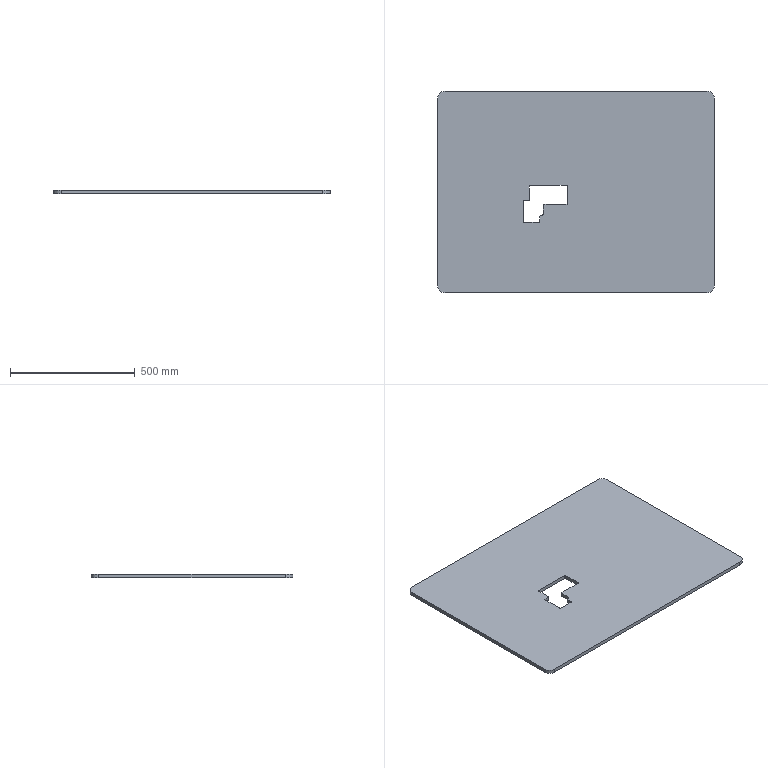Part | SolidWorks | features Cut 1, Extrusion 1 | 1 solid | 31 faces | box 1110 x 810 x 15 mm | volume 13214038 mm3 | plane 17 | cylinder 14 | commonest cylinder face diameters 4 x6 10 x4 60 x4
STEP:
#1=CARTESIAN_POINT('',(-426.754,508.741,0.));
#2=VERTEX_POINT('',#1);
#3=CARTESIAN_POINT('',(-456.754,478.741,0.));
#4=VERTEX_POINT('',#3);
#5=CARTESIAN_POINT('',(-426.754,478.741,0.));
#6=DIRECTION('',(0.,0.,1.));
#7=DIRECTION('',(1.,0.,0.));
#8=AXIS2_PLACEMENT_3D('',#5,#6,#7);
#9=CIRCLE('',#8,30.);
#10=EDGE_CURVE('',#2,#4,#9,.T.);
#11=ORIENTED_EDGE('',*,*,#10,.T.);
#12=CARTESIAN_POINT('',(-456.754,478.741,15.));
#13=VERTEX_POINT('',#12);
#14=CARTESIAN_POINT('',(-456.754,478.741,15.));
#15=DIRECTION('',(0.,0.,-1.));
#16=VECTOR('',#15,1000.);
#17=LINE('',#14,#16);
#18=EDGE_CURVE('',#13,#4,#17,.T.);
#19=ORIENTED_EDGE('',*,*,#18,.F.);
#20=CARTESIAN_POINT('',(-426.754,508.741,15.));
#21=VERTEX_POINT('',#20);
#22=CARTESIAN_POINT('',(-426.754,478.741,15.));
#23=DIRECTION('',(0.,0.,1.));
#24=DIRECTION('',(1.,0.,0.));
#25=AXIS2_PLACEMENT_3D('',#22,#23,#24);
#26=CIRCLE('',#25,30.);
#27=EDGE_CURVE('',#21,#13,#26,.T.);
#28=ORIENTED_EDGE('',*,*,#27,.F.);
#29=CARTESIAN_POINT('',(-426.754,508.741,15.));
#30=DIRECTION('',(0.,0.,-1.));
#31=VECTOR('',#30,1000.);
#32=LINE('',#29,#31);
#33=EDGE_CURVE('',#21,#2,#32,.T.);
#34=ORIENTED_EDGE('',*,*,#33,.T.);
#35=EDGE_LOOP('',(#11,#19,#28,#34));
#36=FACE_OUTER_BOUND('',#35,.T.);
#37=CARTESIAN_POINT('',(-426.754,478.741,15.));
#38=DIRECTION('',(0.,0.,-1.));
#39=DIRECTION('',(-1.,0.,0.));
#40=AXIS2_PLACEMENT_3D('',#37,#38,#39);
#41=CYLINDRICAL_SURFACE('',#40,30.);
#42=ADVANCED_FACE('',(#36),#41,.T.);
#43=CARTESIAN_POINT('',(-456.754,-271.259,0.));
#44=VERTEX_POINT('',#43);
#45=CARTESIAN_POINT('',(-456.754,478.741,0.));
#46=DIRECTION('',(0.,-1.,0.));
#47=VECTOR('',#46,1000.);
#48=LINE('',#45,#47);
#49=EDGE_CURVE('',#4,#44,#48,.T.);
#50=ORIENTED_EDGE('',*,*,#49,.T.);
#51=CARTESIAN_POINT('',(-456.754,-271.259,15.));
#52=VERTEX_POINT('',#51);
#53=CARTESIAN_POINT('',(-456.754,-271.259,15.));
#54=DIRECTION('',(0.,0.,-1.));
#55=VECTOR('',#54,1000.);
#56=LINE('',#53,#55);
#57=EDGE_CURVE('',#52,#44,#56,.T.);
#58=ORIENTED_EDGE('',*,*,#57,.F.);
#59=CARTESIAN_POINT('',(-456.754,478.741,15.));
#60=DIRECTION('',(0.,-1.,0.));
#61=VECTOR('',#60,1000.);
#62=LINE('',#59,#61);
#63=EDGE_CURVE('',#13,#52,#62,.T.);
#64=ORIENTED_EDGE('',*,*,#63,.F.);
#65=ORIENTED_EDGE('',*,*,#18,.T.);
#66=EDGE_LOOP('',(#50,#58,#64,#65));
#67=FACE_OUTER_BOUND('',#66,.T.);
#68=CARTESIAN_POINT('',(-456.754,478.741,15.));
#69=DIRECTION('',(1.,0.,0.));
#70=DIRECTION('',(0.,1.,0.));
#71=AXIS2_PLACEMENT_3D('',#68,#69,#70);
#72=PLANE('',#71);
#73=ADVANCED_FACE('',(#67),#72,.F.);
#74=CARTESIAN_POINT('',(-426.754,-301.259,0.));
#75=VERTEX_POINT('',#74);
#76=CARTESIAN_POINT('',(-426.754,-271.259,0.));
#77=DIRECTION('',(0.,0.,1.));
#78=DIRECTION('',(1.,0.,0.));
#79=AXIS2_PLACEMENT_3D('',#76,#77,#78);
#80=CIRCLE('',#79,30.);
#81=EDGE_CURVE('',#44,#75,#80,.T.);
#82=ORIENTED_EDGE('',*,*,#81,.T.);
#83=CARTESIAN_POINT('',(-426.754,-301.259,15.));
#84=VERTEX_POINT('',#83);
#85=CARTESIAN_POINT('',(-426.754,-301.259,15.));
#86=DIRECTION('',(0.,0.,-1.));
#87=VECTOR('',#86,1000.);
#88=LINE('',#85,#87);
#89=EDGE_CURVE('',#84,#75,#88,.T.);
#90=ORIENTED_EDGE('',*,*,#89,.F.);
#91=CARTESIAN_POINT('',(-426.754,-271.259,15.));
#92=DIRECTION('',(0.,0.,1.));
#93=DIRECTION('',(1.,0.,0.));
#94=AXIS2_PLACEMENT_3D('',#91,#92,#93);
#95=CIRCLE('',#94,30.);
#96=EDGE_CURVE('',#52,#84,#95,.T.);
#97=ORIENTED_EDGE('',*,*,#96,.F.);
#98=ORIENTED_EDGE('',*,*,#57,.T.);
#99=EDGE_LOOP('',(#82,#90,#97,#98));
#100=FACE_OUTER_BOUND('',#99,.T.);
#101=CARTESIAN_POINT('',(-426.754,-271.259,15.));
#102=DIRECTION('',(0.,0.,-1.));
#103=DIRECTION('',(-1.,0.,0.));
#104=AXIS2_PLACEMENT_3D('',#101,#102,#103);
#105=CYLINDRICAL_SURFACE('',#104,30.);
#106=ADVANCED_FACE('',(#100),#105,.T.);
#107=CARTESIAN_POINT('',(623.246,-301.259,0.));
#108=VERTEX_POINT('',#107);
#109=CARTESIAN_POINT('',(623.246,-301.259,0.));
#110=DIRECTION('',(1.,0.,0.));
#111=VECTOR('',#110,1000.);
#112=LINE('',#109,#111);
#113=EDGE_CURVE('',#75,#108,#112,.T.);
#114=ORIENTED_EDGE('',*,*,#113,.T.);
#115=CARTESIAN_POINT('',(623.246,-301.259,15.));
#116=VERTEX_POINT('',#115);
#117=CARTESIAN_POINT('',(623.246,-301.259,15.));
#118=DIRECTION('',(0.,0.,-1.));
#119=VECTOR('',#118,1000.);
#120=LINE('',#117,#119);
#121=EDGE_CURVE('',#116,#108,#120,.T.);
#122=ORIENTED_EDGE('',*,*,#121,.F.);
#123=CARTESIAN_POINT('',(623.246,-301.259,15.));
#124=DIRECTION('',(1.,0.,0.));
#125=VECTOR('',#124,1000.);
#126=LINE('',#123,#125);
#127=EDGE_CURVE('',#84,#116,#126,.T.);
#128=ORIENTED_EDGE('',*,*,#127,.F.);
#129=ORIENTED_EDGE('',*,*,#89,.T.);
#130=EDGE_LOOP('',(#114,#122,#128,#129));
#131=FACE_OUTER_BOUND('',#130,.T.);
#132=CARTESIAN_POINT('',(623.246,-301.259,15.));
#133=DIRECTION('',(0.,1.,0.));
#134=DIRECTION('',(-1.,0.,0.));
#135=AXIS2_PLACEMENT_3D('',#132,#133,#134);
#136=PLANE('',#135);
#137=ADVANCED_FACE('',(#131),#136,.F.);
#138=CARTESIAN_POINT('',(653.246,-271.259,0.));
#139=VERTEX_POINT('',#138);
#140=CARTESIAN_POINT('',(623.246,-271.259,0.));
#141=DIRECTION('',(0.,0.,1.));
#142=DIRECTION('',(1.,0.,0.));
#143=AXIS2_PLACEMENT_3D('',#140,#141,#142);
#144=CIRCLE('',#143,30.);
#145=EDGE_CURVE('',#108,#139,#144,.T.);
#146=ORIENTED_EDGE('',*,*,#145,.T.);
#147=CARTESIAN_POINT('',(653.246,-271.259,15.));
#148=VERTEX_POINT('',#147);
#149=CARTESIAN_POINT('',(653.246,-271.259,15.));
#150=DIRECTION('',(0.,0.,-1.));
#151=VECTOR('',#150,1000.);
#152=LINE('',#149,#151);
#153=EDGE_CURVE('',#148,#139,#152,.T.);
#154=ORIENTED_EDGE('',*,*,#153,.F.);
#155=CARTESIAN_POINT('',(623.246,-271.259,15.));
#156=DIRECTION('',(0.,0.,1.));
#157=DIRECTION('',(1.,0.,0.));
#158=AXIS2_PLACEMENT_3D('',#155,#156,#157);
#159=CIRCLE('',#158,30.);
#160=EDGE_CURVE('',#116,#148,#159,.T.);
#161=ORIENTED_EDGE('',*,*,#160,.F.);
#162=ORIENTED_EDGE('',*,*,#121,.T.);
#163=EDGE_LOOP('',(#146,#154,#161,#162));
#164=FACE_OUTER_BOUND('',#163,.T.);
#165=CARTESIAN_POINT('',(623.246,-271.259,15.));
#166=DIRECTION('',(0.,0.,-1.));
#167=DIRECTION('',(-1.,0.,0.));
#168=AXIS2_PLACEMENT_3D('',#165,#166,#167);
#169=CYLINDRICAL_SURFACE('',#168,30.);
#170=ADVANCED_FACE('',(#164),#169,.T.);
#171=CARTESIAN_POINT('',(653.246,478.741,0.));
#172=VERTEX_POINT('',#171);
#173=CARTESIAN_POINT('',(653.246,478.741,0.));
#174=DIRECTION('',(0.,1.,0.));
#175=VECTOR('',#174,1000.);
#176=LINE('',#173,#175);
#177=EDGE_CURVE('',#139,#172,#176,.T.);
#178=ORIENTED_EDGE('',*,*,#177,.T.);
#179=CARTESIAN_POINT('',(653.246,478.741,15.));
#180=VERTEX_POINT('',#179);
#181=CARTESIAN_POINT('',(653.246,478.741,15.));
#182=DIRECTION('',(0.,0.,-1.));
#183=VECTOR('',#182,1000.);
#184=LINE('',#181,#183);
#185=EDGE_CURVE('',#180,#172,#184,.T.);
#186=ORIENTED_EDGE('',*,*,#185,.F.);
#187=CARTESIAN_POINT('',(653.246,478.741,15.));
#188=DIRECTION('',(0.,1.,0.));
#189=VECTOR('',#188,1000.);
#190=LINE('',#187,#189);
#191=EDGE_CURVE('',#148,#180,#190,.T.);
#192=ORIENTED_EDGE('',*,*,#191,.F.);
#193=ORIENTED_EDGE('',*,*,#153,.T.);
#194=EDGE_LOOP('',(#178,#186,#192,#193));
#195=FACE_OUTER_BOUND('',#194,.T.);
#196=CARTESIAN_POINT('',(653.246,478.741,15.));
#197=DIRECTION('',(-1.,0.,0.));
#198=DIRECTION('',(0.,-1.,0.));
#199=AXIS2_PLACEMENT_3D('',#196,#197,#198);
#200=PLANE('',#199);
#201=ADVANCED_FACE('',(#195),#200,.F.);
#202=CARTESIAN_POINT('',(623.246,508.741,0.));
#203=VERTEX_POINT('',#202);
#204=CARTESIAN_POINT('',(623.246,478.741,0.));
#205=DIRECTION('',(0.,0.,1.));
#206=DIRECTION('',(1.,0.,0.));
#207=AXIS2_PLACEMENT_3D('',#204,#205,#206);
#208=CIRCLE('',#207,30.);
#209=EDGE_CURVE('',#172,#203,#208,.T.);
#210=ORIENTED_EDGE('',*,*,#209,.T.);
#211=CARTESIAN_POINT('',(623.246,508.741,15.));
#212=VERTEX_POINT('',#211);
#213=CARTESIAN_POINT('',(623.246,508.741,15.));
#214=DIRECTION('',(0.,0.,-1.));
#215=VECTOR('',#214,1000.);
#216=LINE('',#213,#215);
#217=EDGE_CURVE('',#212,#203,#216,.T.);
#218=ORIENTED_EDGE('',*,*,#217,.F.);
#219=CARTESIAN_POINT('',(623.246,478.741,15.));
#220=DIRECTION('',(0.,0.,1.));
#221=DIRECTION('',(1.,0.,0.));
#222=AXIS2_PLACEMENT_3D('',#219,#220,#221);
#223=CIRCLE('',#222,30.);
#224=EDGE_CURVE('',#180,#212,#223,.T.);
#225=ORIENTED_EDGE('',*,*,#224,.F.);
#226=ORIENTED_EDGE('',*,*,#185,.T.);
#227=EDGE_LOOP('',(#210,#218,#225,#226));
#228=FACE_OUTER_BOUND('',#227,.T.);
#229=CARTESIAN_POINT('',(623.246,478.741,15.));
#230=DIRECTION('',(0.,0.,-1.));
#231=DIRECTION('',(-1.,0.,0.));
#232=AXIS2_PLACEMENT_3D('',#229,#230,#231);
#233=CYLINDRICAL_SURFACE('',#232,30.);
#234=ADVANCED_FACE('',(#228),#233,.T.);
#235=CARTESIAN_POINT('',(-426.754,508.741,0.));
#236=DIRECTION('',(-1.,0.,0.));
#237=VECTOR('',#236,1000.);
#238=LINE('',#235,#237);
#239=EDGE_CURVE('',#203,#2,#238,.T.);
#240=ORIENTED_EDGE('',*,*,#239,.T.);
#241=ORIENTED_EDGE('',*,*,#33,.F.);
#242=CARTESIAN_POINT('',(-426.754,508.741,15.));
#243=DIRECTION('',(-1.,0.,0.));
#244=VECTOR('',#243,1000.);
#245=LINE('',#242,#244);
#246=EDGE_CURVE('',#212,#21,#245,.T.);
#247=ORIENTED_EDGE('',*,*,#246,.F.);
#248=ORIENTED_EDGE('',*,*,#217,.T.);
#249=EDGE_LOOP('',(#240,#241,#247,#248));
#250=FACE_OUTER_BOUND('',#249,.T.);
#251=CARTESIAN_POINT('',(-426.754,508.741,15.));
#252=DIRECTION('',(0.,-1.,0.));
#253=DIRECTION('',(0.,0.,-1.));
#254=AXIS2_PLACEMENT_3D('',#251,#252,#253);
#255=PLANE('',#254);
#256=ADVANCED_FACE('',(#250),#255,.F.);
#257=CARTESIAN_POINT('',(-20.865,54.676,15.));
#258=VERTEX_POINT('',#257);
#259=CARTESIAN_POINT('',(62.197,54.676,15.));
#260=VERTEX_POINT('',#259);
#261=CARTESIAN_POINT('',(-20.865,54.676,15.));
#262=DIRECTION('',(1.,0.,0.));
#263=VECTOR('',#262,1000.);
#264=LINE('',#261,#263);
#265=EDGE_CURVE('',#258,#260,#264,.T.);
#266=ORIENTED_EDGE('',*,*,#265,.F.);
#267=CARTESIAN_POINT('',(-31.755,54.734,15.));
#268=VERTEX_POINT('',#267);
#269=CARTESIAN_POINT('',(-20.865,54.676,15.));
#270=DIRECTION('',(-1.,0.005339,0.));
#271=VECTOR('',#270,1000.);
#272=LINE('',#269,#271);
#273=EDGE_CURVE('',#258,#268,#272,.T.);
#274=ORIENTED_EDGE('',*,*,#273,.T.);
#275=CARTESIAN_POINT('',(-33.754,53.242,15.));
#276=VERTEX_POINT('',#275);
#277=CARTESIAN_POINT('',(-31.82,52.735,15.));
#278=DIRECTION('',(0.,0.,-1.));
#279=DIRECTION('',(-1.,0.,0.));
#280=AXIS2_PLACEMENT_3D('',#277,#278,#279);
#281=CIRCLE('',#280,2.);
#282=EDGE_CURVE('',#276,#268,#281,.T.);
#283=ORIENTED_EDGE('',*,*,#282,.F.);
#284=CARTESIAN_POINT('',(-33.754,13.803,15.));
#285=VERTEX_POINT('',#284);
#286=CARTESIAN_POINT('',(-33.754,51.678,15.));
#287=DIRECTION('',(0.,1.,0.));
#288=VECTOR('',#287,1000.);
#289=LINE('',#286,#288);
#290=EDGE_CURVE('',#285,#276,#289,.T.);
#291=ORIENTED_EDGE('',*,*,#290,.F.);
#292=CARTESIAN_POINT('',(-38.685,8.804,15.));
#293=VERTEX_POINT('',#292);
#294=CARTESIAN_POINT('',(-38.754,13.803,15.));
#295=DIRECTION('',(0.,0.,-1.));
#296=DIRECTION('',(-1.,0.,0.));
#297=AXIS2_PLACEMENT_3D('',#294,#295,#296);
#298=CIRCLE('',#297,5.);
#299=EDGE_CURVE('',#285,#293,#298,.T.);
#300=ORIENTED_EDGE('',*,*,#299,.T.);
#301=CARTESIAN_POINT('',(-42.824,8.746,15.));
#302=VERTEX_POINT('',#301);
#303=CARTESIAN_POINT('',(-42.824,8.746,15.));
#304=DIRECTION('',(0.9999,0.01383,0.));
#305=VECTOR('',#304,1000.);
#306=LINE('',#303,#305);
#307=EDGE_CURVE('',#302,#293,#306,.T.);
#308=ORIENTED_EDGE('',*,*,#307,.F.);
#309=CARTESIAN_POINT('',(-47.754,3.747,15.));
#310=VERTEX_POINT('',#309);
#311=CARTESIAN_POINT('',(-42.754,3.747,15.));
#312=DIRECTION('',(0.,0.,-1.));
#313=DIRECTION('',(-1.,0.,0.));
#314=AXIS2_PLACEMENT_3D('',#311,#312,#313);
#315=CIRCLE('',#314,5.);
#316=EDGE_CURVE('',#310,#302,#315,.T.);
#317=ORIENTED_EDGE('',*,*,#316,.F.);
#318=CARTESIAN_POINT('',(-47.754,-13.322,15.));
#319=VERTEX_POINT('',#318);
#320=CARTESIAN_POINT('',(-47.754,-13.322,15.));
#321=DIRECTION('',(0.,1.,0.));
#322=VECTOR('',#321,1000.);
#323=LINE('',#320,#322);
#324=EDGE_CURVE('',#319,#310,#323,.T.);
#325=ORIENTED_EDGE('',*,*,#324,.F.);
#326=CARTESIAN_POINT('',(-52.754,-18.322,15.));
#327=VERTEX_POINT('',#326);
#328=CARTESIAN_POINT('',(-52.754,-13.322,15.));
#329=DIRECTION('',(0.,0.,1.));
#330=DIRECTION('',(1.,0.,0.));
#331=AXIS2_PLACEMENT_3D('',#328,#329,#330);
#332=CIRCLE('',#331,5.);
#333=EDGE_CURVE('',#327,#319,#332,.T.);
#334=ORIENTED_EDGE('',*,*,#333,.F.);
#335=CARTESIAN_POINT('',(-108.754,-18.322,15.));
#336=VERTEX_POINT('',#335);
#337=CARTESIAN_POINT('',(-108.754,-18.322,15.));
#338=DIRECTION('',(1.,0.,0.));
#339=VECTOR('',#338,1000.);
#340=LINE('',#337,#339);
#341=EDGE_CURVE('',#336,#327,#340,.T.);
#342=ORIENTED_EDGE('',*,*,#341,.F.);
#343=CARTESIAN_POINT('',(-113.754,-13.322,15.));
#344=VERTEX_POINT('',#343);
#345=CARTESIAN_POINT('',(-108.754,-13.322,15.));
#346=DIRECTION('',(0.,0.,-1.));
#347=DIRECTION('',(-1.,0.,0.));
#348=AXIS2_PLACEMENT_3D('',#345,#346,#347);
#349=CIRCLE('',#348,5.);
#350=EDGE_CURVE('',#336,#344,#349,.T.);
#351=ORIENTED_EDGE('',*,*,#350,.T.);
#352=CARTESIAN_POINT('',(-113.754,68.43,15.));
#353=VERTEX_POINT('',#352);
#354=CARTESIAN_POINT('',(-113.754,51.678,15.));
#355=DIRECTION('',(0.,-1.,0.));
#356=VECTOR('',#355,1000.);
#357=LINE('',#354,#356);
#358=EDGE_CURVE('',#353,#344,#357,.T.);
#359=ORIENTED_EDGE('',*,*,#358,.F.);
#360=CARTESIAN_POINT('',(-111.754,70.43,15.));
#361=VERTEX_POINT('',#360);
#362=CARTESIAN_POINT('',(-111.754,68.43,15.));
#363=DIRECTION('',(0.,0.,-1.));
#364=DIRECTION('',(-1.,0.,0.));
#365=AXIS2_PLACEMENT_3D('',#362,#363,#364);
#366=CIRCLE('',#365,2.);
#367=EDGE_CURVE('',#353,#361,#366,.T.);
#368=ORIENTED_EDGE('',*,*,#367,.T.);
#369=CARTESIAN_POINT('',(-90.692,70.43,15.));
#370=VERTEX_POINT('',#369);
#371=CARTESIAN_POINT('',(-90.692,70.43,15.));
#372=DIRECTION('',(-1.,0.,0.));
#373=VECTOR('',#372,1000.);
#374=LINE('',#371,#373);
#375=EDGE_CURVE('',#370,#361,#374,.T.);
#376=ORIENTED_EDGE('',*,*,#375,.F.);
#377=CARTESIAN_POINT('',(-88.692,72.43,15.));
#378=VERTEX_POINT('',#377);
#379=CARTESIAN_POINT('',(-90.692,72.43,15.));
#380=DIRECTION('',(0.,0.,1.));
#381=DIRECTION('',(1.,0.,0.));
#382=AXIS2_PLACEMENT_3D('',#379,#380,#381);
#383=CIRCLE('',#382,2.);
#384=EDGE_CURVE('',#370,#378,#383,.T.);
#385=ORIENTED_EDGE('',*,*,#384,.T.);
#386=CARTESIAN_POINT('',(-88.692,128.216,15.));
#387=VERTEX_POINT('',#386);
#388=CARTESIAN_POINT('',(-88.692,100.216,15.));
#389=DIRECTION('',(0.,-1.,0.));
#390=VECTOR('',#389,1000.);
#391=LINE('',#388,#390);
#392=EDGE_CURVE('',#387,#378,#391,.T.);
#393=ORIENTED_EDGE('',*,*,#392,.F.);
#394=CARTESIAN_POINT('',(-86.692,130.216,15.));
#395=VERTEX_POINT('',#394);
#396=CARTESIAN_POINT('',(-86.692,128.216,15.));
#397=DIRECTION('',(0.,0.,1.));
#398=DIRECTION('',(1.,0.,0.));
#399=AXIS2_PLACEMENT_3D('',#396,#397,#398);
#400=CIRCLE('',#399,2.);
#401=EDGE_CURVE('',#395,#387,#400,.T.);
#402=ORIENTED_EDGE('',*,*,#401,.F.);
#403=CARTESIAN_POINT('',(62.197,130.216,15.));
#404=VERTEX_POINT('',#403);
#405=CARTESIAN_POINT('',(-86.692,130.216,15.));
#406=DIRECTION('',(1.,0.,0.));
#407=VECTOR('',#406,1000.);
#408=LINE('',#405,#407);
#409=EDGE_CURVE('',#395,#404,#408,.T.);
#410=ORIENTED_EDGE('',*,*,#409,.T.);
#411=CARTESIAN_POINT('',(64.197,128.216,15.));
#412=VERTEX_POINT('',#411);
#413=CARTESIAN_POINT('',(62.197,128.216,15.));
#414=DIRECTION('',(0.,0.,-1.));
#415=DIRECTION('',(-1.,0.,0.));
#416=AXIS2_PLACEMENT_3D('',#413,#414,#415);
#417=CIRCLE('',#416,2.);
#418=EDGE_CURVE('',#404,#412,#417,.T.);
#419=ORIENTED_EDGE('',*,*,#418,.T.);
#420=CARTESIAN_POINT('',(64.197,56.676,15.));
#421=VERTEX_POINT('',#420);
#422=CARTESIAN_POINT('',(64.197,128.216,15.));
#423=DIRECTION('',(0.,-1.,0.));
#424=VECTOR('',#423,1000.);
#425=LINE('',#422,#424);
#426=EDGE_CURVE('',#412,#421,#425,.T.);
#427=ORIENTED_EDGE('',*,*,#426,.T.);
#428=CARTESIAN_POINT('',(62.197,56.676,15.));
#429=DIRECTION('',(0.,0.,1.));
#430=DIRECTION('',(1.,0.,0.));
#431=AXIS2_PLACEMENT_3D('',#428,#429,#430);
#432=CIRCLE('',#431,2.);
#433=EDGE_CURVE('',#260,#421,#432,.T.);
#434=ORIENTED_EDGE('',*,*,#433,.F.);
#435=EDGE_LOOP('',(#266,#274,#283,#291,#300,#308,#317,#325,#334,#342,#351,#359,#368,#376,#385,#393,#402,#410,#419,#427,#434));
#436=FACE_BOUND('',#435,.T.);
#437=ORIENTED_EDGE('',*,*,#27,.T.);
#438=ORIENTED_EDGE('',*,*,#63,.T.);
#439=ORIENTED_EDGE('',*,*,#96,.T.);
#440=ORIENTED_EDGE('',*,*,#127,.T.);
#441=ORIENTED_EDGE('',*,*,#160,.T.);
#442=ORIENTED_EDGE('',*,*,#191,.T.);
#443=ORIENTED_EDGE('',*,*,#224,.T.);
#444=ORIENTED_EDGE('',*,*,#246,.T.);
#445=EDGE_LOOP('',(#437,#438,#439,#440,#441,#442,#443,#444));
#446=FACE_OUTER_BOUND('',#445,.T.);
#447=CARTESIAN_POINT('',(-426.754,478.741,15.));
#448=DIRECTION('',(0.,0.,1.));
#449=DIRECTION('',(1.,0.,0.));
#450=AXIS2_PLACEMENT_3D('',#447,#448,#449);
#451=PLANE('',#450);
#452=ADVANCED_FACE('',(#436,#446),#451,.T.);
#453=CARTESIAN_POINT('',(-20.865,54.676,0.));
#454=VERTEX_POINT('',#453);
#455=CARTESIAN_POINT('',(-31.755,54.734,0.));
#456=VERTEX_POINT('',#455);
#457=CARTESIAN_POINT('',(-20.865,54.676,0.));
#458=DIRECTION('',(-1.,0.005339,0.));
#459=VECTOR('',#458,1000.);
#460=LINE('',#457,#459);
#461=EDGE_CURVE('',#454,#456,#460,.T.);
#462=ORIENTED_EDGE('',*,*,#461,.F.);
#463=CARTESIAN_POINT('',(62.197,54.676,0.));
#464=VERTEX_POINT('',#463);
#465=CARTESIAN_POINT('',(-20.865,54.676,0.));
#466=DIRECTION('',(1.,0.,0.));
#467=VECTOR('',#466,1000.);
#468=LINE('',#465,#467);
#469=EDGE_CURVE('',#454,#464,#468,.T.);
#470=ORIENTED_EDGE('',*,*,#469,.T.);
#471=CARTESIAN_POINT('',(64.197,56.676,0.));
#472=VERTEX_POINT('',#471);
#473=CARTESIAN_POINT('',(62.197,56.676,0.));
#474=DIRECTION('',(0.,0.,1.));
#475=DIRECTION('',(1.,0.,0.));
#476=AXIS2_PLACEMENT_3D('',#473,#474,#475);
#477=CIRCLE('',#476,2.);
#478=EDGE_CURVE('',#464,#472,#477,.T.);
#479=ORIENTED_EDGE('',*,*,#478,.T.);
#480=CARTESIAN_POINT('',(64.197,128.216,0.));
#481=VERTEX_POINT('',#480);
#482=CARTESIAN_POINT('',(64.197,89.976,0.));
#483=DIRECTION('',(0.,-1.,0.));
#484=VECTOR('',#483,1000.);
#485=LINE('',#482,#484);
#486=EDGE_CURVE('',#481,#472,#485,.T.);
#487=ORIENTED_EDGE('',*,*,#486,.F.);
#488=CARTESIAN_POINT('',(62.197,130.216,0.));
#489=VERTEX_POINT('',#488);
#490=CARTESIAN_POINT('',(62.197,128.216,0.));
#491=DIRECTION('',(0.,0.,-1.));
#492=DIRECTION('',(-1.,0.,0.));
#493=AXIS2_PLACEMENT_3D('',#490,#491,#492);
#494=CIRCLE('',#493,2.);
#495=EDGE_CURVE('',#489,#481,#494,.T.);
#496=ORIENTED_EDGE('',*,*,#495,.F.);
#497=CARTESIAN_POINT('',(-86.692,130.216,0.));
#498=VERTEX_POINT('',#497);
#499=CARTESIAN_POINT('',(-86.692,130.216,0.));
#500=DIRECTION('',(1.,0.,0.));
#501=VECTOR('',#500,1000.);
#502=LINE('',#499,#501);
#503=EDGE_CURVE('',#498,#489,#502,.T.);
#504=ORIENTED_EDGE('',*,*,#503,.F.);
#505=CARTESIAN_POINT('',(-88.692,128.216,0.));
#506=VERTEX_POINT('',#505);
#507=CARTESIAN_POINT('',(-86.692,128.216,0.));
#508=DIRECTION('',(0.,0.,1.));
#509=DIRECTION('',(1.,0.,0.));
#510=AXIS2_PLACEMENT_3D('',#507,#508,#509);
#511=CIRCLE('',#510,2.);
#512=EDGE_CURVE('',#498,#506,#511,.T.);
#513=ORIENTED_EDGE('',*,*,#512,.T.);
#514=CARTESIAN_POINT('',(-88.692,72.43,0.));
#515=VERTEX_POINT('',#514);
#516=CARTESIAN_POINT('',(-88.692,100.216,0.));
#517=DIRECTION('',(0.,1.,0.));
#518=VECTOR('',#517,1000.);
#519=LINE('',#516,#518);
#520=EDGE_CURVE('',#515,#506,#519,.T.);
#521=ORIENTED_EDGE('',*,*,#520,.F.);
#522=CARTESIAN_POINT('',(-90.692,70.43,0.));
#523=VERTEX_POINT('',#522);
#524=CARTESIAN_POINT('',(-90.692,72.43,0.));
#525=DIRECTION('',(0.,0.,1.));
#526=DIRECTION('',(1.,0.,0.));
#527=AXIS2_PLACEMENT_3D('',#524,#525,#526);
#528=CIRCLE('',#527,2.);
#529=EDGE_CURVE('',#523,#515,#528,.T.);
#530=ORIENTED_EDGE('',*,*,#529,.F.);
#531=CARTESIAN_POINT('',(-111.754,70.43,0.));
#532=VERTEX_POINT('',#531);
#533=CARTESIAN_POINT('',(-90.692,70.43,0.));
#534=DIRECTION('',(-1.,0.,0.));
#535=VECTOR('',#534,1000.);
#536=LINE('',#533,#535);
#537=EDGE_CURVE('',#523,#532,#536,.T.);
#538=ORIENTED_EDGE('',*,*,#537,.T.);
#539=CARTESIAN_POINT('',(-113.754,68.43,0.));
#540=VERTEX_POINT('',#539);
#541=CARTESIAN_POINT('',(-111.754,68.43,0.));
#542=DIRECTION('',(0.,0.,-1.));
#543=DIRECTION('',(-1.,0.,0.));
#544=AXIS2_PLACEMENT_3D('',#541,#542,#543);
#545=CIRCLE('',#544,2.);
#546=EDGE_CURVE('',#540,#532,#545,.T.);
#547=ORIENTED_EDGE('',*,*,#546,.F.);
#548=CARTESIAN_POINT('',(-113.754,-13.322,0.));
#549=VERTEX_POINT('',#548);
#550=CARTESIAN_POINT('',(-113.754,68.43,0.));
#551=DIRECTION('',(0.,-1.,0.));
#552=VECTOR('',#551,1000.);
#553=LINE('',#550,#552);
#554=EDGE_CURVE('',#540,#549,#553,.T.);
#555=ORIENTED_EDGE('',*,*,#554,.T.);
#556=CARTESIAN_POINT('',(-108.754,-18.322,0.));
#557=VERTEX_POINT('',#556);
#558=CARTESIAN_POINT('',(-108.754,-13.322,0.));
#559=DIRECTION('',(0.,0.,-1.));
#560=DIRECTION('',(-1.,0.,0.));
#561=AXIS2_PLACEMENT_3D('',#558,#559,#560);
#562=CIRCLE('',#561,5.);
#563=EDGE_CURVE('',#557,#549,#562,.T.);
#564=ORIENTED_EDGE('',*,*,#563,.F.);
#565=CARTESIAN_POINT('',(-52.754,-18.322,0.));
#566=VERTEX_POINT('',#565);
#567=CARTESIAN_POINT('',(-108.754,-18.322,0.));
#568=DIRECTION('',(1.,0.,0.));
#569=VECTOR('',#568,1000.);
#570=LINE('',#567,#569);
#571=EDGE_CURVE('',#557,#566,#570,.T.);
#572=ORIENTED_EDGE('',*,*,#571,.T.);
#573=CARTESIAN_POINT('',(-47.754,-13.322,0.));
#574=VERTEX_POINT('',#573);
#575=CARTESIAN_POINT('',(-52.754,-13.322,0.));
#576=DIRECTION('',(0.,0.,1.));
#577=DIRECTION('',(1.,0.,0.));
#578=AXIS2_PLACEMENT_3D('',#575,#576,#577);
#579=CIRCLE('',#578,5.);
#580=EDGE_CURVE('',#566,#574,#579,.T.);
#581=ORIENTED_EDGE('',*,*,#580,.T.);
#582=CARTESIAN_POINT('',(-47.754,3.747,0.));
#583=VERTEX_POINT('',#582);
#584=CARTESIAN_POINT('',(-47.754,-13.322,0.));
#585=DIRECTION('',(0.,1.,0.));
#586=VECTOR('',#585,1000.);
#587=LINE('',#584,#586);
#588=EDGE_CURVE('',#574,#583,#587,.T.);
#589=ORIENTED_EDGE('',*,*,#588,.T.);
#590=CARTESIAN_POINT('',(-42.824,8.746,0.));
#591=VERTEX_POINT('',#590);
#592=CARTESIAN_POINT('',(-42.754,3.747,0.));
#593=DIRECTION('',(0.,0.,-1.));
#594=DIRECTION('',(-1.,0.,0.));
#595=AXIS2_PLACEMENT_3D('',#592,#593,#594);
#596=CIRCLE('',#595,5.);
#597=EDGE_CURVE('',#583,#591,#596,.T.);
#598=ORIENTED_EDGE('',*,*,#597,.T.);
#599=CARTESIAN_POINT('',(-38.685,8.804,0.));
#600=VERTEX_POINT('',#599);
#601=CARTESIAN_POINT('',(-42.824,8.746,0.));
#602=DIRECTION('',(0.9999,0.01383,0.));
#603=VECTOR('',#602,1000.);
#604=LINE('',#601,#603);
#605=EDGE_CURVE('',#591,#600,#604,.T.);
#606=ORIENTED_EDGE('',*,*,#605,.T.);
#607=CARTESIAN_POINT('',(-33.754,13.803,0.));
#608=VERTEX_POINT('',#607);
#609=CARTESIAN_POINT('',(-38.754,13.803,0.));
#610=DIRECTION('',(0.,0.,-1.));
#611=DIRECTION('',(-1.,0.,0.));
#612=AXIS2_PLACEMENT_3D('',#609,#610,#611);
#613=CIRCLE('',#612,5.);
#614=EDGE_CURVE('',#608,#600,#613,.T.);
#615=ORIENTED_EDGE('',*,*,#614,.F.);
#616=CARTESIAN_POINT('',(-33.754,53.242,0.));
#617=VERTEX_POINT('',#616);
#618=CARTESIAN_POINT('',(-33.754,51.678,0.));
#619=DIRECTION('',(0.,-1.,0.));
#620=VECTOR('',#619,1000.);
#621=LINE('',#618,#620);
#622=EDGE_CURVE('',#617,#608,#621,.T.);
#623=ORIENTED_EDGE('',*,*,#622,.F.);
#624=CARTESIAN_POINT('',(-31.82,52.735,0.));
#625=DIRECTION('',(0.,0.,-1.));
#626=DIRECTION('',(-1.,0.,0.));
#627=AXIS2_PLACEMENT_3D('',#624,#625,#626);
#628=CIRCLE('',#627,2.);
#629=EDGE_CURVE('',#617,#456,#628,.T.);
#630=ORIENTED_EDGE('',*,*,#629,.T.);
#631=EDGE_LOOP('',(#462,#470,#479,#487,#496,#504,#513,#521,#530,#538,#547,#555,#564,#572,#581,#589,#598,#606,#615,#623,#630));
#632=FACE_BOUND('',#631,.T.);
#633=ORIENTED_EDGE('',*,*,#10,.F.);
#634=ORIENTED_EDGE('',*,*,#239,.F.);
#635=ORIENTED_EDGE('',*,*,#209,.F.);
#636=ORIENTED_EDGE('',*,*,#177,.F.);
#637=ORIENTED_EDGE('',*,*,#145,.F.);
#638=ORIENTED_EDGE('',*,*,#113,.F.);
#639=ORIENTED_EDGE('',*,*,#81,.F.);
#640=ORIENTED_EDGE('',*,*,#49,.F.);
#641=EDGE_LOOP('',(#633,#634,#635,#636,#637,#638,#639,#640));
#642=FACE_OUTER_BOUND('',#641,.T.);
#643=CARTESIAN_POINT('',(-426.754,478.741,0.));
#644=DIRECTION('',(0.,0.,1.));
#645=DIRECTION('',(1.,0.,0.));
#646=AXIS2_PLACEMENT_3D('',#643,#644,#645);
#647=PLANE('',#646);
#648=ADVANCED_FACE('',(#632,#642),#647,.F.);
#649=ORIENTED_EDGE('',*,*,#265,.T.);
#650=CARTESIAN_POINT('',(62.197,54.676,0.));
#651=DIRECTION('',(0.,0.,1.));
#652=VECTOR('',#651,1000.);
#653=LINE('',#650,#652);
#654=EDGE_CURVE('',#464,#260,#653,.T.);
#655=ORIENTED_EDGE('',*,*,#654,.F.);
#656=ORIENTED_EDGE('',*,*,#469,.F.);
#657=CARTESIAN_POINT('',(-20.865,54.676,0.));
#658=DIRECTION('',(0.,0.,1.));
#659=VECTOR('',#658,1000.);
#660=LINE('',#657,#659);
#661=EDGE_CURVE('',#454,#258,#660,.T.);
#662=ORIENTED_EDGE('',*,*,#661,.T.);
#663=EDGE_LOOP('',(#649,#655,#656,#662));
#664=FACE_OUTER_BOUND('',#663,.T.);
#665=CARTESIAN_POINT('',(-20.865,54.676,0.));
#666=DIRECTION('',(0.,-1.,0.));
#667=DIRECTION('',(0.,0.,-1.));
#668=AXIS2_PLACEMENT_3D('',#665,#666,#667);
#669=PLANE('',#668);
#670=ADVANCED_FACE('',(#664),#669,.F.);
#671=ORIENTED_EDGE('',*,*,#273,.F.);
#672=ORIENTED_EDGE('',*,*,#661,.F.);
#673=ORIENTED_EDGE('',*,*,#461,.T.);
#674=CARTESIAN_POINT('',(-31.755,54.734,0.));
#675=DIRECTION('',(0.,0.,1.));
#676=VECTOR('',#675,1000.);
#677=LINE('',#674,#676);
#678=EDGE_CURVE('',#456,#268,#677,.T.);
#679=ORIENTED_EDGE('',*,*,#678,.T.);
#680=EDGE_LOOP('',(#671,#672,#673,#679));
#681=FACE_OUTER_BOUND('',#680,.T.);
#682=CARTESIAN_POINT('',(-20.865,54.676,0.));
#683=DIRECTION('',(0.005339,1.,0.));
#684=DIRECTION('',(-1.,0.005339,0.));
#685=AXIS2_PLACEMENT_3D('',#682,#683,#684);
#686=PLANE('',#685);
#687=ADVANCED_FACE('',(#681),#686,.T.);
#688=ORIENTED_EDGE('',*,*,#282,.T.);
#689=ORIENTED_EDGE('',*,*,#678,.F.);
#690=ORIENTED_EDGE('',*,*,#629,.F.);
#691=CARTESIAN_POINT('',(-33.754,53.242,0.));
#692=DIRECTION('',(0.,0.,1.));
#693=VECTOR('',#692,1000.);
#694=LINE('',#691,#693);
#695=EDGE_CURVE('',#617,#276,#694,.T.);
#696=ORIENTED_EDGE('',*,*,#695,.T.);
#697=EDGE_LOOP('',(#688,#689,#690,#696));
#698=FACE_OUTER_BOUND('',#697,.T.);
#699=CARTESIAN_POINT('',(-31.82,52.735,0.));
#700=DIRECTION('',(0.,0.,1.));
#701=DIRECTION('',(1.,0.,0.));
#702=AXIS2_PLACEMENT_3D('',#699,#700,#701);
#703=CYLINDRICAL_SURFACE('',#702,2.);
#704=ADVANCED_FACE('',(#698),#703,.T.);
#705=ORIENTED_EDGE('',*,*,#290,.T.);
#706=ORIENTED_EDGE('',*,*,#695,.F.);
#707=ORIENTED_EDGE('',*,*,#622,.T.);
#708=CARTESIAN_POINT('',(-33.754,13.803,0.));
#709=DIRECTION('',(0.,0.,1.));
#710=VECTOR('',#709,1000.);
#711=LINE('',#708,#710);
#712=EDGE_CURVE('',#608,#285,#711,.T.);
#713=ORIENTED_EDGE('',*,*,#712,.T.);
#714=EDGE_LOOP('',(#705,#706,#707,#713));
#715=FACE_OUTER_BOUND('',#714,.T.);
#716=CARTESIAN_POINT('',(-33.754,51.678,0.));
#717=DIRECTION('',(1.,0.,0.));
#718=DIRECTION('',(0.,0.,-1.));
#719=AXIS2_PLACEMENT_3D('',#716,#717,#718);
#720=PLANE('',#719);
#721=ADVANCED_FACE('',(#715),#720,.F.);
#722=ORIENTED_EDGE('',*,*,#299,.F.);
#723=ORIENTED_EDGE('',*,*,#712,.F.);
#724=ORIENTED_EDGE('',*,*,#614,.T.);
#725=CARTESIAN_POINT('',(-38.685,8.804,0.));
#726=DIRECTION('',(0.,0.,1.));
#727=VECTOR('',#726,1000.);
#728=LINE('',#725,#727);
#729=EDGE_CURVE('',#600,#293,#728,.T.);
#730=ORIENTED_EDGE('',*,*,#729,.T.);
#731=EDGE_LOOP('',(#722,#723,#724,#730));
#732=FACE_OUTER_BOUND('',#731,.T.);
#733=CARTESIAN_POINT('',(-38.754,13.803,0.));
#734=DIRECTION('',(0.,0.,1.));
#735=DIRECTION('',(1.,0.,0.));
#736=AXIS2_PLACEMENT_3D('',#733,#734,#735);
#737=CYLINDRICAL_SURFACE('',#736,5.);
#738=ADVANCED_FACE('',(#732),#737,.F.);
#739=ORIENTED_EDGE('',*,*,#307,.T.);
#740=ORIENTED_EDGE('',*,*,#729,.F.);
#741=ORIENTED_EDGE('',*,*,#605,.F.);
#742=CARTESIAN_POINT('',(-42.824,8.746,0.));
#743=DIRECTION('',(0.,0.,1.));
#744=VECTOR('',#743,1000.);
#745=LINE('',#742,#744);
#746=EDGE_CURVE('',#591,#302,#745,.T.);
#747=ORIENTED_EDGE('',*,*,#746,.T.);
#748=EDGE_LOOP('',(#739,#740,#741,#747));
#749=FACE_OUTER_BOUND('',#748,.T.);
#750=CARTESIAN_POINT('',(-42.824,8.746,0.));
#751=DIRECTION('',(0.01383,-0.9999,0.));
#752=DIRECTION('',(0.9999,0.01383,0.));
#753=AXIS2_PLACEMENT_3D('',#750,#751,#752);
#754=PLANE('',#753);
#755=ADVANCED_FACE('',(#749),#754,.F.);
#756=ORIENTED_EDGE('',*,*,#316,.T.);
#757=ORIENTED_EDGE('',*,*,#746,.F.);
#758=ORIENTED_EDGE('',*,*,#597,.F.);
#759=CARTESIAN_POINT('',(-47.754,3.747,0.));
#760=DIRECTION('',(0.,0.,1.));
#761=VECTOR('',#760,1000.);
#762=LINE('',#759,#761);
#763=EDGE_CURVE('',#583,#310,#762,.T.);
#764=ORIENTED_EDGE('',*,*,#763,.T.);
#765=EDGE_LOOP('',(#756,#757,#758,#764));
#766=FACE_OUTER_BOUND('',#765,.T.);
#767=CARTESIAN_POINT('',(-42.754,3.747,0.));
#768=DIRECTION('',(0.,0.,1.));
#769=DIRECTION('',(1.,0.,0.));
#770=AXIS2_PLACEMENT_3D('',#767,#768,#769);
#771=CYLINDRICAL_SURFACE('',#770,5.);
#772=ADVANCED_FACE('',(#766),#771,.T.);
#773=ORIENTED_EDGE('',*,*,#324,.T.);
#774=ORIENTED_EDGE('',*,*,#763,.F.);
#775=ORIENTED_EDGE('',*,*,#588,.F.);
#776=CARTESIAN_POINT('',(-47.754,-13.322,0.));
#777=DIRECTION('',(0.,0.,1.));
#778=VECTOR('',#777,1000.);
#779=LINE('',#776,#778);
#780=EDGE_CURVE('',#574,#319,#779,.T.);
#781=ORIENTED_EDGE('',*,*,#780,.T.);
#782=EDGE_LOOP('',(#773,#774,#775,#781));
#783=FACE_OUTER_BOUND('',#782,.T.);
#784=CARTESIAN_POINT('',(-47.754,-13.322,0.));
#785=DIRECTION('',(1.,0.,0.));
#786=DIRECTION('',(0.,0.,-1.));
#787=AXIS2_PLACEMENT_3D('',#784,#785,#786);
#788=PLANE('',#787);
#789=ADVANCED_FACE('',(#783),#788,.F.);
#790=ORIENTED_EDGE('',*,*,#333,.T.);
#791=ORIENTED_EDGE('',*,*,#780,.F.);
#792=ORIENTED_EDGE('',*,*,#580,.F.);
#793=CARTESIAN_POINT('',(-52.754,-18.322,0.));
#794=DIRECTION('',(0.,0.,1.));
#795=VECTOR('',#794,1000.);
#796=LINE('',#793,#795);
#797=EDGE_CURVE('',#566,#327,#796,.T.);
#798=ORIENTED_EDGE('',*,*,#797,.T.);
#799=EDGE_LOOP('',(#790,#791,#792,#798));
#800=FACE_OUTER_BOUND('',#799,.T.);
#801=CARTESIAN_POINT('',(-52.754,-13.322,0.));
#802=DIRECTION('',(0.,0.,1.));
#803=DIRECTION('',(1.,0.,0.));
#804=AXIS2_PLACEMENT_3D('',#801,#802,#803);
#805=CYLINDRICAL_SURFACE('',#804,5.);
#806=ADVANCED_FACE('',(#800),#805,.F.);
#807=ORIENTED_EDGE('',*,*,#341,.T.);
#808=ORIENTED_EDGE('',*,*,#797,.F.);
#809=ORIENTED_EDGE('',*,*,#571,.F.);
#810=CARTESIAN_POINT('',(-108.754,-18.322,0.));
#811=DIRECTION('',(0.,0.,1.));
#812=VECTOR('',#811,1000.);
#813=LINE('',#810,#812);
#814=EDGE_CURVE('',#557,#336,#813,.T.);
#815=ORIENTED_EDGE('',*,*,#814,.T.);
#816=EDGE_LOOP('',(#807,#808,#809,#815));
#817=FACE_OUTER_BOUND('',#816,.T.);
#818=CARTESIAN_POINT('',(-108.754,-18.322,0.));
#819=DIRECTION('',(0.,-1.,0.));
#820=DIRECTION('',(0.,0.,-1.));
#821=AXIS2_PLACEMENT_3D('',#818,#819,#820);
#822=PLANE('',#821);
#823=ADVANCED_FACE('',(#817),#822,.F.);
#824=ORIENTED_EDGE('',*,*,#350,.F.);
#825=ORIENTED_EDGE('',*,*,#814,.F.);
#826=ORIENTED_EDGE('',*,*,#563,.T.);
#827=CARTESIAN_POINT('',(-113.754,-13.322,0.));
#828=DIRECTION('',(0.,0.,1.));
#829=VECTOR('',#828,1000.);
#830=LINE('',#827,#829);
#831=EDGE_CURVE('',#549,#344,#830,.T.);
#832=ORIENTED_EDGE('',*,*,#831,.T.);
#833=EDGE_LOOP('',(#824,#825,#826,#832));
#834=FACE_OUTER_BOUND('',#833,.T.);
#835=CARTESIAN_POINT('',(-108.754,-13.322,0.));
#836=DIRECTION('',(0.,0.,1.));
#837=DIRECTION('',(1.,0.,0.));
#838=AXIS2_PLACEMENT_3D('',#835,#836,#837);
#839=CYLINDRICAL_SURFACE('',#838,5.);
#840=ADVANCED_FACE('',(#834),#839,.F.);
#841=ORIENTED_EDGE('',*,*,#358,.T.);
#842=ORIENTED_EDGE('',*,*,#831,.F.);
#843=ORIENTED_EDGE('',*,*,#554,.F.);
#844=CARTESIAN_POINT('',(-113.754,68.43,0.));
#845=DIRECTION('',(0.,0.,1.));
#846=VECTOR('',#845,1000.);
#847=LINE('',#844,#846);
#848=EDGE_CURVE('',#540,#353,#847,.T.);
#849=ORIENTED_EDGE('',*,*,#848,.T.);
#850=EDGE_LOOP('',(#841,#842,#843,#849));
#851=FACE_OUTER_BOUND('',#850,.T.);
#852=CARTESIAN_POINT('',(-113.754,51.678,0.));
#853=DIRECTION('',(-1.,0.,0.));
#854=DIRECTION('',(0.,0.,1.));
#855=AXIS2_PLACEMENT_3D('',#852,#853,#854);
#856=PLANE('',#855);
#857=ADVANCED_FACE('',(#851),#856,.F.);
#858=ORIENTED_EDGE('',*,*,#367,.F.);
#859=ORIENTED_EDGE('',*,*,#848,.F.);
#860=ORIENTED_EDGE('',*,*,#546,.T.);
#861=CARTESIAN_POINT('',(-111.754,70.43,0.));
#862=DIRECTION('',(0.,0.,1.));
#863=VECTOR('',#862,1000.);
#864=LINE('',#861,#863);
#865=EDGE_CURVE('',#532,#361,#864,.T.);
#866=ORIENTED_EDGE('',*,*,#865,.T.);
#867=EDGE_LOOP('',(#858,#859,#860,#866));
#868=FACE_OUTER_BOUND('',#867,.T.);
#869=CARTESIAN_POINT('',(-111.754,68.43,0.));
#870=DIRECTION('',(0.,0.,1.));
#871=DIRECTION('',(1.,0.,0.));
#872=AXIS2_PLACEMENT_3D('',#869,#870,#871);
#873=CYLINDRICAL_SURFACE('',#872,2.);
#874=ADVANCED_FACE('',(#868),#873,.F.);
#875=ORIENTED_EDGE('',*,*,#375,.T.);
#876=ORIENTED_EDGE('',*,*,#865,.F.);
#877=ORIENTED_EDGE('',*,*,#537,.F.);
#878=CARTESIAN_POINT('',(-90.692,70.43,0.));
#879=DIRECTION('',(0.,0.,1.));
#880=VECTOR('',#879,1000.);
#881=LINE('',#878,#880);
#882=EDGE_CURVE('',#523,#370,#881,.T.);
#883=ORIENTED_EDGE('',*,*,#882,.T.);
#884=EDGE_LOOP('',(#875,#876,#877,#883));
#885=FACE_OUTER_BOUND('',#884,.T.);
#886=CARTESIAN_POINT('',(-90.692,70.43,0.));
#887=DIRECTION('',(0.,1.,0.));
#888=DIRECTION('',(0.,0.,1.));
#889=AXIS2_PLACEMENT_3D('',#886,#887,#888);
#890=PLANE('',#889);
#891=ADVANCED_FACE('',(#885),#890,.F.);
#892=ORIENTED_EDGE('',*,*,#384,.F.);
#893=ORIENTED_EDGE('',*,*,#882,.F.);
#894=ORIENTED_EDGE('',*,*,#529,.T.);
#895=CARTESIAN_POINT('',(-88.692,72.43,0.));
#896=DIRECTION('',(0.,0.,1.));
#897=VECTOR('',#896,1000.);
#898=LINE('',#895,#897);
#899=EDGE_CURVE('',#515,#378,#898,.T.);
#900=ORIENTED_EDGE('',*,*,#899,.T.);
#901=EDGE_LOOP('',(#892,#893,#894,#900));
#902=FACE_OUTER_BOUND('',#901,.T.);
#903=CARTESIAN_POINT('',(-90.692,72.43,0.));
#904=DIRECTION('',(0.,0.,1.));
#905=DIRECTION('',(1.,0.,0.));
#906=AXIS2_PLACEMENT_3D('',#903,#904,#905);
#907=CYLINDRICAL_SURFACE('',#906,2.);
#908=ADVANCED_FACE('',(#902),#907,.T.);
#909=ORIENTED_EDGE('',*,*,#392,.T.);
#910=ORIENTED_EDGE('',*,*,#899,.F.);
#911=ORIENTED_EDGE('',*,*,#520,.T.);
#912=CARTESIAN_POINT('',(-88.692,128.216,0.));
#913=DIRECTION('',(0.,0.,1.));
#914=VECTOR('',#913,1000.);
#915=LINE('',#912,#914);
#916=EDGE_CURVE('',#506,#387,#915,.T.);
#917=ORIENTED_EDGE('',*,*,#916,.T.);
#918=EDGE_LOOP('',(#909,#910,#911,#917));
#919=FACE_OUTER_BOUND('',#918,.T.);
#920=CARTESIAN_POINT('',(-88.692,100.216,0.));
#921=DIRECTION('',(-1.,0.,0.));
#922=DIRECTION('',(0.,0.,1.));
#923=AXIS2_PLACEMENT_3D('',#920,#921,#922);
#924=PLANE('',#923);
#925=ADVANCED_FACE('',(#919),#924,.F.);
#926=ORIENTED_EDGE('',*,*,#401,.T.);
#927=ORIENTED_EDGE('',*,*,#916,.F.);
#928=ORIENTED_EDGE('',*,*,#512,.F.);
#929=CARTESIAN_POINT('',(-86.692,130.216,0.));
#930=DIRECTION('',(0.,0.,1.));
#931=VECTOR('',#930,1000.);
#932=LINE('',#929,#931);
#933=EDGE_CURVE('',#498,#395,#932,.T.);
#934=ORIENTED_EDGE('',*,*,#933,.T.);
#935=EDGE_LOOP('',(#926,#927,#928,#934));
#936=FACE_OUTER_BOUND('',#935,.T.);
#937=CARTESIAN_POINT('',(-86.692,128.216,0.));
#938=DIRECTION('',(0.,0.,1.));
#939=DIRECTION('',(1.,0.,0.));
#940=AXIS2_PLACEMENT_3D('',#937,#938,#939);
#941=CYLINDRICAL_SURFACE('',#940,2.);
#942=ADVANCED_FACE('',(#936),#941,.F.);
#943=ORIENTED_EDGE('',*,*,#409,.F.);
#944=ORIENTED_EDGE('',*,*,#933,.F.);
#945=ORIENTED_EDGE('',*,*,#503,.T.);
#946=CARTESIAN_POINT('',(62.197,130.216,0.));
#947=DIRECTION('',(0.,0.,1.));
#948=VECTOR('',#947,1000.);
#949=LINE('',#946,#948);
#950=EDGE_CURVE('',#489,#404,#949,.T.);
#951=ORIENTED_EDGE('',*,*,#950,.T.);
#952=EDGE_LOOP('',(#943,#944,#945,#951));
#953=FACE_OUTER_BOUND('',#952,.T.);
#954=CARTESIAN_POINT('',(-86.692,130.216,0.));
#955=DIRECTION('',(0.,-1.,0.));
#956=DIRECTION('',(0.,0.,-1.));
#957=AXIS2_PLACEMENT_3D('',#954,#955,#956);
#958=PLANE('',#957);
#959=ADVANCED_FACE('',(#953),#958,.T.);
#960=ORIENTED_EDGE('',*,*,#418,.F.);
#961=ORIENTED_EDGE('',*,*,#950,.F.);
#962=ORIENTED_EDGE('',*,*,#495,.T.);
#963=CARTESIAN_POINT('',(64.197,128.216,0.));
#964=DIRECTION('',(0.,0.,1.));
#965=VECTOR('',#964,1000.);
#966=LINE('',#963,#965);
#967=EDGE_CURVE('',#481,#412,#966,.T.);
#968=ORIENTED_EDGE('',*,*,#967,.T.);
#969=EDGE_LOOP('',(#960,#961,#962,#968));
#970=FACE_OUTER_BOUND('',#969,.T.);
#971=CARTESIAN_POINT('',(62.197,128.216,0.));
#972=DIRECTION('',(0.,0.,1.));
#973=DIRECTION('',(1.,0.,0.));
#974=AXIS2_PLACEMENT_3D('',#971,#972,#973);
#975=CYLINDRICAL_SURFACE('',#974,2.);
#976=ADVANCED_FACE('',(#970),#975,.F.);
#977=ORIENTED_EDGE('',*,*,#426,.F.);
#978=ORIENTED_EDGE('',*,*,#967,.F.);
#979=ORIENTED_EDGE('',*,*,#486,.T.);
#980=CARTESIAN_POINT('',(64.197,56.676,0.));
#981=DIRECTION('',(0.,0.,1.));
#982=VECTOR('',#981,1000.);
#983=LINE('',#980,#982);
#984=EDGE_CURVE('',#472,#421,#983,.T.);
#985=ORIENTED_EDGE('',*,*,#984,.T.);
#986=EDGE_LOOP('',(#977,#978,#979,#985));
#987=FACE_OUTER_BOUND('',#986,.T.);
#988=CARTESIAN_POINT('',(64.197,128.216,0.));
#989=DIRECTION('',(-1.,0.,0.));
#990=DIRECTION('',(0.,0.,1.));
#991=AXIS2_PLACEMENT_3D('',#988,#989,#990);
#992=PLANE('',#991);
#993=ADVANCED_FACE('',(#987),#992,.T.);
#994=ORIENTED_EDGE('',*,*,#433,.T.);
#995=ORIENTED_EDGE('',*,*,#984,.F.);
#996=ORIENTED_EDGE('',*,*,#478,.F.);
#997=ORIENTED_EDGE('',*,*,#654,.T.);
#998=EDGE_LOOP('',(#994,#995,#996,#997));
#999=FACE_OUTER_BOUND('',#998,.T.);
#1000=CARTESIAN_POINT('',(62.197,56.676,0.));
#1001=DIRECTION('',(0.,0.,1.));
#1002=DIRECTION('',(1.,0.,0.));
#1003=AXIS2_PLACEMENT_3D('',#1000,#1001,#1002);
#1004=CYLINDRICAL_SURFACE('',#1003,2.);
#1005=ADVANCED_FACE('',(#999),#1004,.F.);
#1006=CLOSED_SHELL('',(#42,#73,#106,#137,#170,#201,#234,#256,#452,#648,#670,#687,#704,#721,#738,#755,#772,#789,#806,#823,#840,#857,#874,#891,#908,#925,#942,#959,#976,#993,#1005));
#1007=MANIFOLD_SOLID_BREP('',#1006);
#1008=CARTESIAN_POINT('',(0.,0.,0.));
#1009=DIRECTION('',(0.,0.,1.));
#1010=DIRECTION('',(1.,0.,0.));
#1011=AXIS2_PLACEMENT_3D('',#1008,#1009,#1010);
#1012=(LENGTH_UNIT()NAMED_UNIT(*)SI_UNIT(.MILLI.,.METRE.));
#1013=UNCERTAINTY_MEASURE_WITH_UNIT(LENGTH_MEASURE(0.00001),#1012,'','');
#1014=(NAMED_UNIT(*)PLANE_ANGLE_UNIT()SI_UNIT($,.RADIAN.));
#1015=(NAMED_UNIT(*)SI_UNIT($,.STERADIAN.)SOLID_ANGLE_UNIT());
#1016=(GEOMETRIC_REPRESENTATION_CONTEXT(3)GLOBAL_UNCERTAINTY_ASSIGNED_CONTEXT((#1013))GLOBAL_UNIT_ASSIGNED_CONTEXT((#1012,#1014,#1015))REPRESENTATION_CONTEXT('',''));
#1017=ADVANCED_BREP_SHAPE_REPRESENTATION('',(#1007,#1011),#1016);